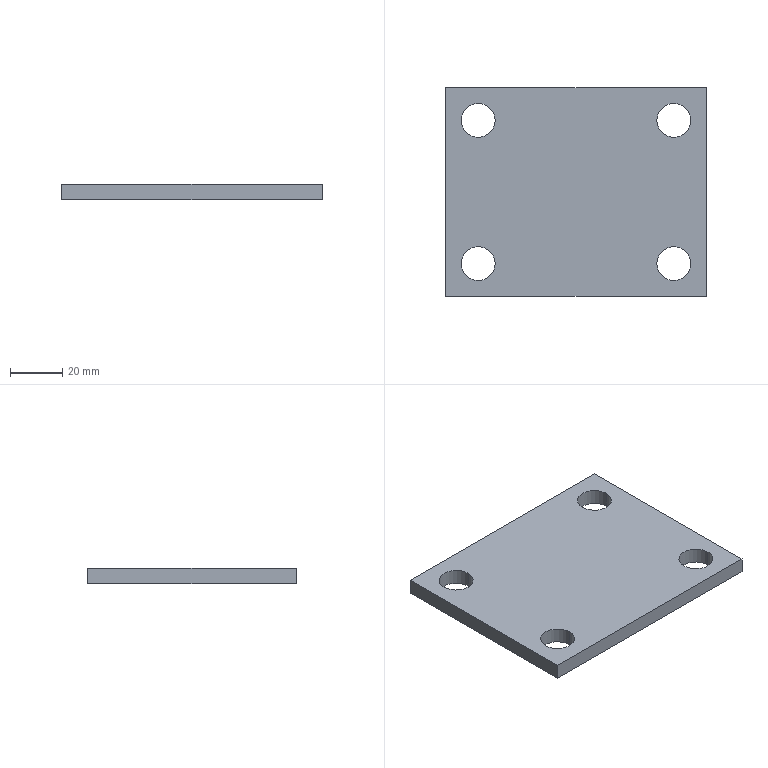Part | SolidWorks | features Extrusion 1, ICE 1 | 1 solid | 14 faces | box 100 x 80 x 6 mm | volume 44814 mm3 | cylinder 8 | plane 6 | commonest cylinder face diameters 13 x8
STEP:
#1=CARTESIAN_POINT('',(-44.,-27.5,0.));
#2=VERTEX_POINT('',#1);
#3=CARTESIAN_POINT('',(-31.,-27.5,0.));
#4=VERTEX_POINT('',#3);
#5=CARTESIAN_POINT('',(-37.5,-27.5,0.));
#6=DIRECTION('',(0.,0.,1.));
#7=DIRECTION('',(1.,0.,0.));
#8=AXIS2_PLACEMENT_3D('',#5,#6,#7);
#9=CIRCLE('',#8,6.5);
#10=EDGE_CURVE('',#2,#4,#9,.T.);
#11=ORIENTED_EDGE('',*,*,#10,.F.);
#12=CARTESIAN_POINT('',(-44.,-27.5,6.));
#13=VERTEX_POINT('',#12);
#14=CARTESIAN_POINT('',(-44.,-27.5,0.));
#15=DIRECTION('',(0.,0.,1.));
#16=VECTOR('',#15,1000.);
#17=LINE('',#14,#16);
#18=EDGE_CURVE('',#2,#13,#17,.T.);
#19=ORIENTED_EDGE('',*,*,#18,.T.);
#20=CARTESIAN_POINT('',(-31.,-27.5,6.));
#21=VERTEX_POINT('',#20);
#22=CARTESIAN_POINT('',(-37.5,-27.5,6.));
#23=DIRECTION('',(0.,0.,1.));
#24=DIRECTION('',(1.,0.,0.));
#25=AXIS2_PLACEMENT_3D('',#22,#23,#24);
#26=CIRCLE('',#25,6.5);
#27=EDGE_CURVE('',#13,#21,#26,.T.);
#28=ORIENTED_EDGE('',*,*,#27,.T.);
#29=CARTESIAN_POINT('',(-31.,-27.5,0.));
#30=DIRECTION('',(0.,0.,1.));
#31=VECTOR('',#30,1000.);
#32=LINE('',#29,#31);
#33=EDGE_CURVE('',#4,#21,#32,.T.);
#34=ORIENTED_EDGE('',*,*,#33,.F.);
#35=EDGE_LOOP('',(#11,#19,#28,#34));
#36=FACE_OUTER_BOUND('',#35,.T.);
#37=CARTESIAN_POINT('',(-37.5,-27.5,0.));
#38=DIRECTION('',(0.,0.,1.));
#39=DIRECTION('',(1.,0.,0.));
#40=AXIS2_PLACEMENT_3D('',#37,#38,#39);
#41=CYLINDRICAL_SURFACE('',#40,6.5);
#42=ADVANCED_FACE('',(#36),#41,.F.);
#43=CARTESIAN_POINT('',(31.,-27.5,0.));
#44=VERTEX_POINT('',#43);
#45=CARTESIAN_POINT('',(44.,-27.5,0.));
#46=VERTEX_POINT('',#45);
#47=CARTESIAN_POINT('',(37.5,-27.5,0.));
#48=DIRECTION('',(0.,0.,1.));
#49=DIRECTION('',(1.,0.,0.));
#50=AXIS2_PLACEMENT_3D('',#47,#48,#49);
#51=CIRCLE('',#50,6.5);
#52=EDGE_CURVE('',#44,#46,#51,.T.);
#53=ORIENTED_EDGE('',*,*,#52,.F.);
#54=CARTESIAN_POINT('',(31.,-27.5,6.));
#55=VERTEX_POINT('',#54);
#56=CARTESIAN_POINT('',(31.,-27.5,0.));
#57=DIRECTION('',(0.,0.,1.));
#58=VECTOR('',#57,1000.);
#59=LINE('',#56,#58);
#60=EDGE_CURVE('',#44,#55,#59,.T.);
#61=ORIENTED_EDGE('',*,*,#60,.T.);
#62=CARTESIAN_POINT('',(44.,-27.5,6.));
#63=VERTEX_POINT('',#62);
#64=CARTESIAN_POINT('',(37.5,-27.5,6.));
#65=DIRECTION('',(0.,0.,1.));
#66=DIRECTION('',(1.,0.,0.));
#67=AXIS2_PLACEMENT_3D('',#64,#65,#66);
#68=CIRCLE('',#67,6.5);
#69=EDGE_CURVE('',#55,#63,#68,.T.);
#70=ORIENTED_EDGE('',*,*,#69,.T.);
#71=CARTESIAN_POINT('',(44.,-27.5,0.));
#72=DIRECTION('',(0.,0.,1.));
#73=VECTOR('',#72,1000.);
#74=LINE('',#71,#73);
#75=EDGE_CURVE('',#46,#63,#74,.T.);
#76=ORIENTED_EDGE('',*,*,#75,.F.);
#77=EDGE_LOOP('',(#53,#61,#70,#76));
#78=FACE_OUTER_BOUND('',#77,.T.);
#79=CARTESIAN_POINT('',(37.5,-27.5,0.));
#80=DIRECTION('',(0.,0.,1.));
#81=DIRECTION('',(1.,0.,0.));
#82=AXIS2_PLACEMENT_3D('',#79,#80,#81);
#83=CYLINDRICAL_SURFACE('',#82,6.5);
#84=ADVANCED_FACE('',(#78),#83,.F.);
#85=CARTESIAN_POINT('',(31.,27.5,0.));
#86=VERTEX_POINT('',#85);
#87=CARTESIAN_POINT('',(44.,27.5,0.));
#88=VERTEX_POINT('',#87);
#89=CARTESIAN_POINT('',(37.5,27.5,0.));
#90=DIRECTION('',(0.,0.,1.));
#91=DIRECTION('',(1.,0.,0.));
#92=AXIS2_PLACEMENT_3D('',#89,#90,#91);
#93=CIRCLE('',#92,6.5);
#94=EDGE_CURVE('',#86,#88,#93,.T.);
#95=ORIENTED_EDGE('',*,*,#94,.F.);
#96=CARTESIAN_POINT('',(31.,27.5,6.));
#97=VERTEX_POINT('',#96);
#98=CARTESIAN_POINT('',(31.,27.5,0.));
#99=DIRECTION('',(0.,0.,1.));
#100=VECTOR('',#99,1000.);
#101=LINE('',#98,#100);
#102=EDGE_CURVE('',#86,#97,#101,.T.);
#103=ORIENTED_EDGE('',*,*,#102,.T.);
#104=CARTESIAN_POINT('',(44.,27.5,6.));
#105=VERTEX_POINT('',#104);
#106=CARTESIAN_POINT('',(37.5,27.5,6.));
#107=DIRECTION('',(0.,0.,1.));
#108=DIRECTION('',(1.,0.,0.));
#109=AXIS2_PLACEMENT_3D('',#106,#107,#108);
#110=CIRCLE('',#109,6.5);
#111=EDGE_CURVE('',#97,#105,#110,.T.);
#112=ORIENTED_EDGE('',*,*,#111,.T.);
#113=CARTESIAN_POINT('',(44.,27.5,0.));
#114=DIRECTION('',(0.,0.,1.));
#115=VECTOR('',#114,1000.);
#116=LINE('',#113,#115);
#117=EDGE_CURVE('',#88,#105,#116,.T.);
#118=ORIENTED_EDGE('',*,*,#117,.F.);
#119=EDGE_LOOP('',(#95,#103,#112,#118));
#120=FACE_OUTER_BOUND('',#119,.T.);
#121=CARTESIAN_POINT('',(37.5,27.5,0.));
#122=DIRECTION('',(0.,0.,1.));
#123=DIRECTION('',(1.,0.,0.));
#124=AXIS2_PLACEMENT_3D('',#121,#122,#123);
#125=CYLINDRICAL_SURFACE('',#124,6.5);
#126=ADVANCED_FACE('',(#120),#125,.F.);
#127=CARTESIAN_POINT('',(-44.,27.5,0.));
#128=VERTEX_POINT('',#127);
#129=CARTESIAN_POINT('',(-31.,27.5,0.));
#130=VERTEX_POINT('',#129);
#131=CARTESIAN_POINT('',(-37.5,27.5,0.));
#132=DIRECTION('',(0.,0.,1.));
#133=DIRECTION('',(1.,0.,0.));
#134=AXIS2_PLACEMENT_3D('',#131,#132,#133);
#135=CIRCLE('',#134,6.5);
#136=EDGE_CURVE('',#128,#130,#135,.T.);
#137=ORIENTED_EDGE('',*,*,#136,.F.);
#138=CARTESIAN_POINT('',(-44.,27.5,6.));
#139=VERTEX_POINT('',#138);
#140=CARTESIAN_POINT('',(-44.,27.5,0.));
#141=DIRECTION('',(0.,0.,1.));
#142=VECTOR('',#141,1000.);
#143=LINE('',#140,#142);
#144=EDGE_CURVE('',#128,#139,#143,.T.);
#145=ORIENTED_EDGE('',*,*,#144,.T.);
#146=CARTESIAN_POINT('',(-31.,27.5,6.));
#147=VERTEX_POINT('',#146);
#148=CARTESIAN_POINT('',(-37.5,27.5,6.));
#149=DIRECTION('',(0.,0.,1.));
#150=DIRECTION('',(1.,0.,0.));
#151=AXIS2_PLACEMENT_3D('',#148,#149,#150);
#152=CIRCLE('',#151,6.5);
#153=EDGE_CURVE('',#139,#147,#152,.T.);
#154=ORIENTED_EDGE('',*,*,#153,.T.);
#155=CARTESIAN_POINT('',(-31.,27.5,0.));
#156=DIRECTION('',(0.,0.,1.));
#157=VECTOR('',#156,1000.);
#158=LINE('',#155,#157);
#159=EDGE_CURVE('',#130,#147,#158,.T.);
#160=ORIENTED_EDGE('',*,*,#159,.F.);
#161=EDGE_LOOP('',(#137,#145,#154,#160));
#162=FACE_OUTER_BOUND('',#161,.T.);
#163=CARTESIAN_POINT('',(-37.5,27.5,0.));
#164=DIRECTION('',(0.,0.,1.));
#165=DIRECTION('',(1.,0.,0.));
#166=AXIS2_PLACEMENT_3D('',#163,#164,#165);
#167=CYLINDRICAL_SURFACE('',#166,6.5);
#168=ADVANCED_FACE('',(#162),#167,.F.);
#169=CARTESIAN_POINT('',(-50.,40.,0.));
#170=VERTEX_POINT('',#169);
#171=CARTESIAN_POINT('',(-50.,-40.,0.));
#172=VERTEX_POINT('',#171);
#173=CARTESIAN_POINT('',(-50.,40.,0.));
#174=DIRECTION('',(0.,-1.,0.));
#175=VECTOR('',#174,1000.);
#176=LINE('',#173,#175);
#177=EDGE_CURVE('',#170,#172,#176,.T.);
#178=ORIENTED_EDGE('',*,*,#177,.T.);
#179=CARTESIAN_POINT('',(-50.,-40.,6.));
#180=VERTEX_POINT('',#179);
#181=CARTESIAN_POINT('',(-50.,-40.,6.));
#182=DIRECTION('',(0.,0.,-1.));
#183=VECTOR('',#182,1000.);
#184=LINE('',#181,#183);
#185=EDGE_CURVE('',#180,#172,#184,.T.);
#186=ORIENTED_EDGE('',*,*,#185,.F.);
#187=CARTESIAN_POINT('',(-50.,40.,6.));
#188=VERTEX_POINT('',#187);
#189=CARTESIAN_POINT('',(-50.,40.,6.));
#190=DIRECTION('',(0.,-1.,0.));
#191=VECTOR('',#190,1000.);
#192=LINE('',#189,#191);
#193=EDGE_CURVE('',#188,#180,#192,.T.);
#194=ORIENTED_EDGE('',*,*,#193,.F.);
#195=CARTESIAN_POINT('',(-50.,40.,6.));
#196=DIRECTION('',(0.,0.,-1.));
#197=VECTOR('',#196,1000.);
#198=LINE('',#195,#197);
#199=EDGE_CURVE('',#188,#170,#198,.T.);
#200=ORIENTED_EDGE('',*,*,#199,.T.);
#201=EDGE_LOOP('',(#178,#186,#194,#200));
#202=FACE_OUTER_BOUND('',#201,.T.);
#203=CARTESIAN_POINT('',(-50.,40.,6.));
#204=DIRECTION('',(1.,0.,0.));
#205=DIRECTION('',(0.,1.,0.));
#206=AXIS2_PLACEMENT_3D('',#203,#204,#205);
#207=PLANE('',#206);
#208=ADVANCED_FACE('',(#202),#207,.F.);
#209=CARTESIAN_POINT('',(50.,-40.,0.));
#210=VERTEX_POINT('',#209);
#211=CARTESIAN_POINT('',(50.,-40.,0.));
#212=DIRECTION('',(1.,0.,0.));
#213=VECTOR('',#212,1000.);
#214=LINE('',#211,#213);
#215=EDGE_CURVE('',#172,#210,#214,.T.);
#216=ORIENTED_EDGE('',*,*,#215,.T.);
#217=CARTESIAN_POINT('',(50.,-40.,6.));
#218=VERTEX_POINT('',#217);
#219=CARTESIAN_POINT('',(50.,-40.,6.));
#220=DIRECTION('',(0.,0.,-1.));
#221=VECTOR('',#220,1000.);
#222=LINE('',#219,#221);
#223=EDGE_CURVE('',#218,#210,#222,.T.);
#224=ORIENTED_EDGE('',*,*,#223,.F.);
#225=CARTESIAN_POINT('',(50.,-40.,6.));
#226=DIRECTION('',(1.,0.,0.));
#227=VECTOR('',#226,1000.);
#228=LINE('',#225,#227);
#229=EDGE_CURVE('',#180,#218,#228,.T.);
#230=ORIENTED_EDGE('',*,*,#229,.F.);
#231=ORIENTED_EDGE('',*,*,#185,.T.);
#232=EDGE_LOOP('',(#216,#224,#230,#231));
#233=FACE_OUTER_BOUND('',#232,.T.);
#234=CARTESIAN_POINT('',(50.,-40.,6.));
#235=DIRECTION('',(0.,1.,0.));
#236=DIRECTION('',(-1.,0.,0.));
#237=AXIS2_PLACEMENT_3D('',#234,#235,#236);
#238=PLANE('',#237);
#239=ADVANCED_FACE('',(#233),#238,.F.);
#240=CARTESIAN_POINT('',(50.,40.,0.));
#241=VERTEX_POINT('',#240);
#242=CARTESIAN_POINT('',(50.,40.,0.));
#243=DIRECTION('',(0.,1.,0.));
#244=VECTOR('',#243,1000.);
#245=LINE('',#242,#244);
#246=EDGE_CURVE('',#210,#241,#245,.T.);
#247=ORIENTED_EDGE('',*,*,#246,.T.);
#248=CARTESIAN_POINT('',(50.,40.,6.));
#249=VERTEX_POINT('',#248);
#250=CARTESIAN_POINT('',(50.,40.,6.));
#251=DIRECTION('',(0.,0.,-1.));
#252=VECTOR('',#251,1000.);
#253=LINE('',#250,#252);
#254=EDGE_CURVE('',#249,#241,#253,.T.);
#255=ORIENTED_EDGE('',*,*,#254,.F.);
#256=CARTESIAN_POINT('',(50.,40.,6.));
#257=DIRECTION('',(0.,1.,0.));
#258=VECTOR('',#257,1000.);
#259=LINE('',#256,#258);
#260=EDGE_CURVE('',#218,#249,#259,.T.);
#261=ORIENTED_EDGE('',*,*,#260,.F.);
#262=ORIENTED_EDGE('',*,*,#223,.T.);
#263=EDGE_LOOP('',(#247,#255,#261,#262));
#264=FACE_OUTER_BOUND('',#263,.T.);
#265=CARTESIAN_POINT('',(50.,40.,6.));
#266=DIRECTION('',(-1.,0.,0.));
#267=DIRECTION('',(0.,-1.,0.));
#268=AXIS2_PLACEMENT_3D('',#265,#266,#267);
#269=PLANE('',#268);
#270=ADVANCED_FACE('',(#264),#269,.F.);
#271=CARTESIAN_POINT('',(50.,40.,0.));
#272=DIRECTION('',(-1.,0.,0.));
#273=VECTOR('',#272,1000.);
#274=LINE('',#271,#273);
#275=EDGE_CURVE('',#241,#170,#274,.T.);
#276=ORIENTED_EDGE('',*,*,#275,.T.);
#277=ORIENTED_EDGE('',*,*,#199,.F.);
#278=CARTESIAN_POINT('',(50.,40.,6.));
#279=DIRECTION('',(-1.,0.,0.));
#280=VECTOR('',#279,1000.);
#281=LINE('',#278,#280);
#282=EDGE_CURVE('',#249,#188,#281,.T.);
#283=ORIENTED_EDGE('',*,*,#282,.F.);
#284=ORIENTED_EDGE('',*,*,#254,.T.);
#285=EDGE_LOOP('',(#276,#277,#283,#284));
#286=FACE_OUTER_BOUND('',#285,.T.);
#287=CARTESIAN_POINT('',(50.,40.,6.));
#288=DIRECTION('',(0.,-1.,0.));
#289=DIRECTION('',(1.,0.,0.));
#290=AXIS2_PLACEMENT_3D('',#287,#288,#289);
#291=PLANE('',#290);
#292=ADVANCED_FACE('',(#286),#291,.F.);
#293=CARTESIAN_POINT('',(-37.5,-27.5,6.));
#294=DIRECTION('',(0.,0.,1.));
#295=DIRECTION('',(1.,0.,0.));
#296=AXIS2_PLACEMENT_3D('',#293,#294,#295);
#297=CIRCLE('',#296,6.5);
#298=EDGE_CURVE('',#21,#13,#297,.T.);
#299=ORIENTED_EDGE('',*,*,#298,.F.);
#300=ORIENTED_EDGE('',*,*,#27,.F.);
#301=EDGE_LOOP('',(#299,#300));
#302=FACE_BOUND('',#301,.T.);
#303=CARTESIAN_POINT('',(37.5,-27.5,6.));
#304=DIRECTION('',(0.,0.,1.));
#305=DIRECTION('',(1.,0.,0.));
#306=AXIS2_PLACEMENT_3D('',#303,#304,#305);
#307=CIRCLE('',#306,6.5);
#308=EDGE_CURVE('',#63,#55,#307,.T.);
#309=ORIENTED_EDGE('',*,*,#308,.F.);
#310=ORIENTED_EDGE('',*,*,#69,.F.);
#311=EDGE_LOOP('',(#309,#310));
#312=FACE_BOUND('',#311,.T.);
#313=CARTESIAN_POINT('',(37.5,27.5,6.));
#314=DIRECTION('',(0.,0.,1.));
#315=DIRECTION('',(1.,0.,0.));
#316=AXIS2_PLACEMENT_3D('',#313,#314,#315);
#317=CIRCLE('',#316,6.5);
#318=EDGE_CURVE('',#105,#97,#317,.T.);
#319=ORIENTED_EDGE('',*,*,#318,.F.);
#320=ORIENTED_EDGE('',*,*,#111,.F.);
#321=EDGE_LOOP('',(#319,#320));
#322=FACE_BOUND('',#321,.T.);
#323=CARTESIAN_POINT('',(-37.5,27.5,6.));
#324=DIRECTION('',(0.,0.,1.));
#325=DIRECTION('',(1.,0.,0.));
#326=AXIS2_PLACEMENT_3D('',#323,#324,#325);
#327=CIRCLE('',#326,6.5);
#328=EDGE_CURVE('',#147,#139,#327,.T.);
#329=ORIENTED_EDGE('',*,*,#328,.F.);
#330=ORIENTED_EDGE('',*,*,#153,.F.);
#331=EDGE_LOOP('',(#329,#330));
#332=FACE_BOUND('',#331,.T.);
#333=ORIENTED_EDGE('',*,*,#193,.T.);
#334=ORIENTED_EDGE('',*,*,#229,.T.);
#335=ORIENTED_EDGE('',*,*,#260,.T.);
#336=ORIENTED_EDGE('',*,*,#282,.T.);
#337=EDGE_LOOP('',(#333,#334,#335,#336));
#338=FACE_OUTER_BOUND('',#337,.T.);
#339=CARTESIAN_POINT('',(0.,0.,6.));
#340=DIRECTION('',(0.,0.,-1.));
#341=DIRECTION('',(-1.,0.,0.));
#342=AXIS2_PLACEMENT_3D('',#339,#340,#341);
#343=PLANE('',#342);
#344=ADVANCED_FACE('',(#302,#312,#322,#332,#338),#343,.F.);
#345=CARTESIAN_POINT('',(-37.5,-27.5,0.));
#346=DIRECTION('',(0.,0.,1.));
#347=DIRECTION('',(1.,0.,0.));
#348=AXIS2_PLACEMENT_3D('',#345,#346,#347);
#349=CIRCLE('',#348,6.5);
#350=EDGE_CURVE('',#4,#2,#349,.T.);
#351=ORIENTED_EDGE('',*,*,#350,.T.);
#352=ORIENTED_EDGE('',*,*,#10,.T.);
#353=EDGE_LOOP('',(#351,#352));
#354=FACE_BOUND('',#353,.T.);
#355=CARTESIAN_POINT('',(37.5,-27.5,0.));
#356=DIRECTION('',(0.,0.,1.));
#357=DIRECTION('',(1.,0.,0.));
#358=AXIS2_PLACEMENT_3D('',#355,#356,#357);
#359=CIRCLE('',#358,6.5);
#360=EDGE_CURVE('',#46,#44,#359,.T.);
#361=ORIENTED_EDGE('',*,*,#360,.T.);
#362=ORIENTED_EDGE('',*,*,#52,.T.);
#363=EDGE_LOOP('',(#361,#362));
#364=FACE_BOUND('',#363,.T.);
#365=CARTESIAN_POINT('',(37.5,27.5,0.));
#366=DIRECTION('',(0.,0.,1.));
#367=DIRECTION('',(1.,0.,0.));
#368=AXIS2_PLACEMENT_3D('',#365,#366,#367);
#369=CIRCLE('',#368,6.5);
#370=EDGE_CURVE('',#88,#86,#369,.T.);
#371=ORIENTED_EDGE('',*,*,#370,.T.);
#372=ORIENTED_EDGE('',*,*,#94,.T.);
#373=EDGE_LOOP('',(#371,#372));
#374=FACE_BOUND('',#373,.T.);
#375=CARTESIAN_POINT('',(-37.5,27.5,0.));
#376=DIRECTION('',(0.,0.,1.));
#377=DIRECTION('',(1.,0.,0.));
#378=AXIS2_PLACEMENT_3D('',#375,#376,#377);
#379=CIRCLE('',#378,6.5);
#380=EDGE_CURVE('',#130,#128,#379,.T.);
#381=ORIENTED_EDGE('',*,*,#380,.T.);
#382=ORIENTED_EDGE('',*,*,#136,.T.);
#383=EDGE_LOOP('',(#381,#382));
#384=FACE_BOUND('',#383,.T.);
#385=ORIENTED_EDGE('',*,*,#177,.F.);
#386=ORIENTED_EDGE('',*,*,#275,.F.);
#387=ORIENTED_EDGE('',*,*,#246,.F.);
#388=ORIENTED_EDGE('',*,*,#215,.F.);
#389=EDGE_LOOP('',(#385,#386,#387,#388));
#390=FACE_OUTER_BOUND('',#389,.T.);
#391=CARTESIAN_POINT('',(0.,0.,0.));
#392=DIRECTION('',(0.,0.,-1.));
#393=DIRECTION('',(-1.,0.,0.));
#394=AXIS2_PLACEMENT_3D('',#391,#392,#393);
#395=PLANE('',#394);
#396=ADVANCED_FACE('',(#354,#364,#374,#384,#390),#395,.T.);
#397=ORIENTED_EDGE('',*,*,#144,.F.);
#398=ORIENTED_EDGE('',*,*,#380,.F.);
#399=ORIENTED_EDGE('',*,*,#159,.T.);
#400=ORIENTED_EDGE('',*,*,#328,.T.);
#401=EDGE_LOOP('',(#397,#398,#399,#400));
#402=FACE_OUTER_BOUND('',#401,.T.);
#403=CARTESIAN_POINT('',(-37.5,27.5,0.));
#404=DIRECTION('',(0.,0.,1.));
#405=DIRECTION('',(1.,0.,0.));
#406=AXIS2_PLACEMENT_3D('',#403,#404,#405);
#407=CYLINDRICAL_SURFACE('',#406,6.5);
#408=ADVANCED_FACE('',(#402),#407,.F.);
#409=ORIENTED_EDGE('',*,*,#102,.F.);
#410=ORIENTED_EDGE('',*,*,#370,.F.);
#411=ORIENTED_EDGE('',*,*,#117,.T.);
#412=ORIENTED_EDGE('',*,*,#318,.T.);
#413=EDGE_LOOP('',(#409,#410,#411,#412));
#414=FACE_OUTER_BOUND('',#413,.T.);
#415=CARTESIAN_POINT('',(37.5,27.5,0.));
#416=DIRECTION('',(0.,0.,1.));
#417=DIRECTION('',(1.,0.,0.));
#418=AXIS2_PLACEMENT_3D('',#415,#416,#417);
#419=CYLINDRICAL_SURFACE('',#418,6.5);
#420=ADVANCED_FACE('',(#414),#419,.F.);
#421=ORIENTED_EDGE('',*,*,#60,.F.);
#422=ORIENTED_EDGE('',*,*,#360,.F.);
#423=ORIENTED_EDGE('',*,*,#75,.T.);
#424=ORIENTED_EDGE('',*,*,#308,.T.);
#425=EDGE_LOOP('',(#421,#422,#423,#424));
#426=FACE_OUTER_BOUND('',#425,.T.);
#427=CARTESIAN_POINT('',(37.5,-27.5,0.));
#428=DIRECTION('',(0.,0.,1.));
#429=DIRECTION('',(1.,0.,0.));
#430=AXIS2_PLACEMENT_3D('',#427,#428,#429);
#431=CYLINDRICAL_SURFACE('',#430,6.5);
#432=ADVANCED_FACE('',(#426),#431,.F.);
#433=ORIENTED_EDGE('',*,*,#18,.F.);
#434=ORIENTED_EDGE('',*,*,#350,.F.);
#435=ORIENTED_EDGE('',*,*,#33,.T.);
#436=ORIENTED_EDGE('',*,*,#298,.T.);
#437=EDGE_LOOP('',(#433,#434,#435,#436));
#438=FACE_OUTER_BOUND('',#437,.T.);
#439=CARTESIAN_POINT('',(-37.5,-27.5,0.));
#440=DIRECTION('',(0.,0.,1.));
#441=DIRECTION('',(1.,0.,0.));
#442=AXIS2_PLACEMENT_3D('',#439,#440,#441);
#443=CYLINDRICAL_SURFACE('',#442,6.5);
#444=ADVANCED_FACE('',(#438),#443,.F.);
#445=CLOSED_SHELL('',(#42,#84,#126,#168,#208,#239,#270,#292,#344,#396,#408,#420,#432,#444));
#446=MANIFOLD_SOLID_BREP('',#445);
#447=CARTESIAN_POINT('',(0.,0.,0.));
#448=DIRECTION('',(0.,0.,1.));
#449=DIRECTION('',(1.,0.,0.));
#450=AXIS2_PLACEMENT_3D('',#447,#448,#449);
#451=(LENGTH_UNIT()NAMED_UNIT(*)SI_UNIT(.MILLI.,.METRE.));
#452=UNCERTAINTY_MEASURE_WITH_UNIT(LENGTH_MEASURE(0.00001),#451,'','');
#453=(NAMED_UNIT(*)PLANE_ANGLE_UNIT()SI_UNIT($,.RADIAN.));
#454=(NAMED_UNIT(*)SI_UNIT($,.STERADIAN.)SOLID_ANGLE_UNIT());
#455=(GEOMETRIC_REPRESENTATION_CONTEXT(3)GLOBAL_UNCERTAINTY_ASSIGNED_CONTEXT((#452))GLOBAL_UNIT_ASSIGNED_CONTEXT((#451,#453,#454))REPRESENTATION_CONTEXT('',''));
#456=ADVANCED_BREP_SHAPE_REPRESENTATION('',(#446,#450),#455);